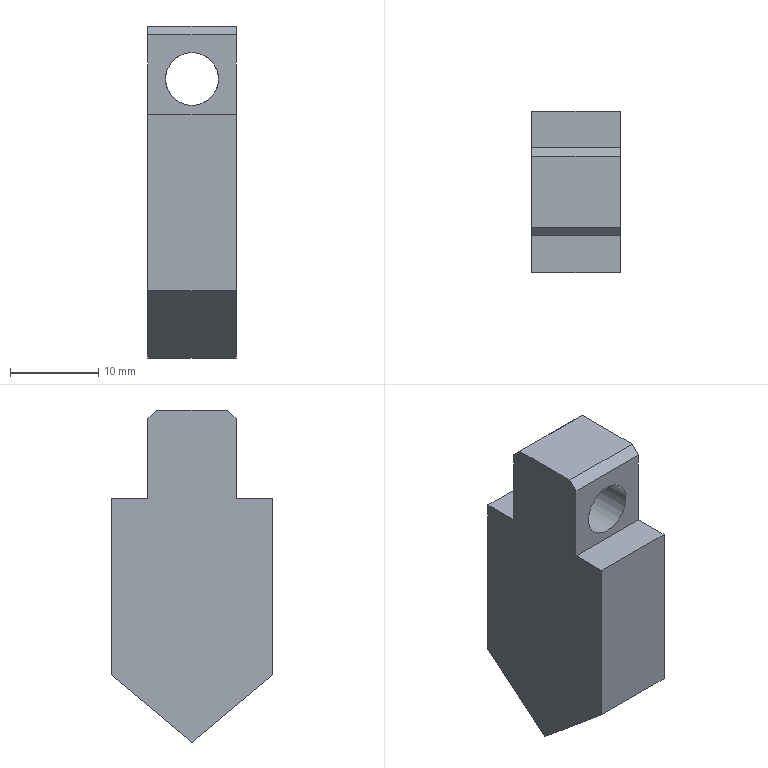Part | NX | features DATUM_CSYS 3, CHAMFER 2, EXTRUDE 2, SKETCH 2 | 1 solid | 14 faces | box 10 x 18.2 x 37.6 mm | volume 5039 mm3 | plane 13 | cylinder 1 | commonest cylinder face diameters 6 x1
STEP:
#1=CARTESIAN_POINT('',(0.,-9.1,27.6));
#2=VERTEX_POINT('',#1);
#3=CARTESIAN_POINT('',(0.,-9.1,7.6));
#4=VERTEX_POINT('',#3);
#5=CARTESIAN_POINT('',(0.,-9.1,27.6));
#6=DIRECTION('',(0.,0.,-1.));
#7=VECTOR('',#6,1000.);
#8=LINE('',#5,#7);
#9=EDGE_CURVE('',#2,#4,#8,.T.);
#10=ORIENTED_EDGE('',*,*,#9,.T.);
#11=CARTESIAN_POINT('',(10.,-9.1,7.6));
#12=VERTEX_POINT('',#11);
#13=CARTESIAN_POINT('',(10.,-9.1,7.6));
#14=DIRECTION('',(-1.,0.,0.));
#15=VECTOR('',#14,1000.);
#16=LINE('',#13,#15);
#17=EDGE_CURVE('',#12,#4,#16,.T.);
#18=ORIENTED_EDGE('',*,*,#17,.F.);
#19=CARTESIAN_POINT('',(10.,-9.1,27.6));
#20=VERTEX_POINT('',#19);
#21=CARTESIAN_POINT('',(10.,-9.1,27.6));
#22=DIRECTION('',(0.,0.,-1.));
#23=VECTOR('',#22,1000.);
#24=LINE('',#21,#23);
#25=EDGE_CURVE('',#20,#12,#24,.T.);
#26=ORIENTED_EDGE('',*,*,#25,.F.);
#27=CARTESIAN_POINT('',(10.,-9.1,27.6));
#28=DIRECTION('',(-1.,0.,0.));
#29=VECTOR('',#28,1000.);
#30=LINE('',#27,#29);
#31=EDGE_CURVE('',#20,#2,#30,.T.);
#32=ORIENTED_EDGE('',*,*,#31,.T.);
#33=EDGE_LOOP('',(#10,#18,#26,#32));
#34=FACE_BOUND('',#33,.T.);
#35=CARTESIAN_POINT('',(10.,-9.1,27.6));
#36=DIRECTION('',(0.,1.,0.));
#37=DIRECTION('',(0.,0.,1.));
#38=AXIS2_PLACEMENT_3D('',#35,#36,#37);
#39=PLANE('',#38);
#40=ADVANCED_FACE('',(#34),#39,.F.);
#41=CARTESIAN_POINT('',(0.,0.,0.));
#42=VERTEX_POINT('',#41);
#43=CARTESIAN_POINT('',(0.,-9.1,7.6));
#44=DIRECTION('',(0.,0.7675,-0.641));
#45=VECTOR('',#44,1000.);
#46=LINE('',#43,#45);
#47=EDGE_CURVE('',#4,#42,#46,.T.);
#48=ORIENTED_EDGE('',*,*,#47,.T.);
#49=CARTESIAN_POINT('',(10.,0.,0.));
#50=VERTEX_POINT('',#49);
#51=CARTESIAN_POINT('',(10.,0.,0.));
#52=DIRECTION('',(-1.,0.,0.));
#53=VECTOR('',#52,1000.);
#54=LINE('',#51,#53);
#55=EDGE_CURVE('',#50,#42,#54,.T.);
#56=ORIENTED_EDGE('',*,*,#55,.F.);
#57=CARTESIAN_POINT('',(10.,-9.1,7.6));
#58=DIRECTION('',(0.,0.7675,-0.641));
#59=VECTOR('',#58,1000.);
#60=LINE('',#57,#59);
#61=EDGE_CURVE('',#12,#50,#60,.T.);
#62=ORIENTED_EDGE('',*,*,#61,.F.);
#63=ORIENTED_EDGE('',*,*,#17,.T.);
#64=EDGE_LOOP('',(#48,#56,#62,#63));
#65=FACE_BOUND('',#64,.T.);
#66=CARTESIAN_POINT('',(10.,-9.1,7.6));
#67=DIRECTION('',(0.,0.641,0.7675));
#68=DIRECTION('',(0.,-0.7675,0.641));
#69=AXIS2_PLACEMENT_3D('',#66,#67,#68);
#70=PLANE('',#69);
#71=ADVANCED_FACE('',(#65),#70,.F.);
#72=CARTESIAN_POINT('',(0.,9.1,7.6));
#73=VERTEX_POINT('',#72);
#74=CARTESIAN_POINT('',(0.,0.,0.));
#75=DIRECTION('',(0.,0.7675,0.641));
#76=VECTOR('',#75,1000.);
#77=LINE('',#74,#76);
#78=EDGE_CURVE('',#42,#73,#77,.T.);
#79=ORIENTED_EDGE('',*,*,#78,.T.);
#80=CARTESIAN_POINT('',(10.,9.1,7.6));
#81=VERTEX_POINT('',#80);
#82=CARTESIAN_POINT('',(10.,9.1,7.6));
#83=DIRECTION('',(-1.,0.,0.));
#84=VECTOR('',#83,1000.);
#85=LINE('',#82,#84);
#86=EDGE_CURVE('',#81,#73,#85,.T.);
#87=ORIENTED_EDGE('',*,*,#86,.F.);
#88=CARTESIAN_POINT('',(10.,0.,0.));
#89=DIRECTION('',(0.,0.7675,0.641));
#90=VECTOR('',#89,1000.);
#91=LINE('',#88,#90);
#92=EDGE_CURVE('',#50,#81,#91,.T.);
#93=ORIENTED_EDGE('',*,*,#92,.F.);
#94=ORIENTED_EDGE('',*,*,#55,.T.);
#95=EDGE_LOOP('',(#79,#87,#93,#94));
#96=FACE_BOUND('',#95,.T.);
#97=CARTESIAN_POINT('',(10.,0.,0.));
#98=DIRECTION('',(0.,-0.641,0.7675));
#99=DIRECTION('',(0.,-0.7675,-0.641));
#100=AXIS2_PLACEMENT_3D('',#97,#98,#99);
#101=PLANE('',#100);
#102=ADVANCED_FACE('',(#96),#101,.F.);
#103=CARTESIAN_POINT('',(0.,9.1,27.6));
#104=VERTEX_POINT('',#103);
#105=CARTESIAN_POINT('',(0.,9.1,7.6));
#106=DIRECTION('',(0.,0.,1.));
#107=VECTOR('',#106,1000.);
#108=LINE('',#105,#107);
#109=EDGE_CURVE('',#73,#104,#108,.T.);
#110=ORIENTED_EDGE('',*,*,#109,.T.);
#111=CARTESIAN_POINT('',(10.,9.1,27.6));
#112=VERTEX_POINT('',#111);
#113=CARTESIAN_POINT('',(10.,9.1,27.6));
#114=DIRECTION('',(-1.,0.,0.));
#115=VECTOR('',#114,1000.);
#116=LINE('',#113,#115);
#117=EDGE_CURVE('',#112,#104,#116,.T.);
#118=ORIENTED_EDGE('',*,*,#117,.F.);
#119=CARTESIAN_POINT('',(10.,9.1,7.6));
#120=DIRECTION('',(0.,0.,1.));
#121=VECTOR('',#120,1000.);
#122=LINE('',#119,#121);
#123=EDGE_CURVE('',#81,#112,#122,.T.);
#124=ORIENTED_EDGE('',*,*,#123,.F.);
#125=ORIENTED_EDGE('',*,*,#86,.T.);
#126=EDGE_LOOP('',(#110,#118,#124,#125));
#127=FACE_BOUND('',#126,.T.);
#128=CARTESIAN_POINT('',(10.,9.1,7.6));
#129=DIRECTION('',(0.,-1.,0.));
#130=DIRECTION('',(0.,0.,-1.));
#131=AXIS2_PLACEMENT_3D('',#128,#129,#130);
#132=PLANE('',#131);
#133=ADVANCED_FACE('',(#127),#132,.F.);
#134=CARTESIAN_POINT('',(0.,5.,27.6));
#135=VERTEX_POINT('',#134);
#136=CARTESIAN_POINT('',(0.,9.1,27.6));
#137=DIRECTION('',(0.,-1.,0.));
#138=VECTOR('',#137,1000.);
#139=LINE('',#136,#138);
#140=EDGE_CURVE('',#104,#135,#139,.T.);
#141=ORIENTED_EDGE('',*,*,#140,.T.);
#142=CARTESIAN_POINT('',(10.,5.,27.6));
#143=VERTEX_POINT('',#142);
#144=CARTESIAN_POINT('',(10.,5.,27.6));
#145=DIRECTION('',(-1.,0.,0.));
#146=VECTOR('',#145,1000.);
#147=LINE('',#144,#146);
#148=EDGE_CURVE('',#143,#135,#147,.T.);
#149=ORIENTED_EDGE('',*,*,#148,.F.);
#150=CARTESIAN_POINT('',(10.,9.1,27.6));
#151=DIRECTION('',(0.,-1.,0.));
#152=VECTOR('',#151,1000.);
#153=LINE('',#150,#152);
#154=EDGE_CURVE('',#112,#143,#153,.T.);
#155=ORIENTED_EDGE('',*,*,#154,.F.);
#156=ORIENTED_EDGE('',*,*,#117,.T.);
#157=EDGE_LOOP('',(#141,#149,#155,#156));
#158=FACE_BOUND('',#157,.T.);
#159=CARTESIAN_POINT('',(10.,9.1,27.6));
#160=DIRECTION('',(0.,0.,-1.));
#161=DIRECTION('',(-1.,0.,0.));
#162=AXIS2_PLACEMENT_3D('',#159,#160,#161);
#163=PLANE('',#162);
#164=ADVANCED_FACE('',(#158),#163,.F.);
#165=CARTESIAN_POINT('',(2.,5.,31.6));
#166=VERTEX_POINT('',#165);
#167=CARTESIAN_POINT('',(5.,5.,31.6));
#168=DIRECTION('',(0.,1.,0.));
#169=DIRECTION('',(-1.,0.,0.));
#170=AXIS2_PLACEMENT_3D('',#167,#168,#169);
#171=CIRCLE('',#170,3.);
#172=EDGE_CURVE('',#166,#166,#171,.T.);
#173=ORIENTED_EDGE('',*,*,#172,.F.);
#174=EDGE_LOOP('',(#173));
#175=FACE_BOUND('',#174,.T.);
#176=CARTESIAN_POINT('',(0.,5.,36.6));
#177=VERTEX_POINT('',#176);
#178=CARTESIAN_POINT('',(0.,5.,27.6));
#179=DIRECTION('',(0.,0.,1.));
#180=VECTOR('',#179,1000.);
#181=LINE('',#178,#180);
#182=EDGE_CURVE('',#135,#177,#181,.T.);
#183=ORIENTED_EDGE('',*,*,#182,.T.);
#184=CARTESIAN_POINT('',(10.,5.,36.6));
#185=VERTEX_POINT('',#184);
#186=CARTESIAN_POINT('',(10.,5.,36.6));
#187=DIRECTION('',(1.,0.,0.));
#188=VECTOR('',#187,1000.);
#189=LINE('',#186,#188);
#190=EDGE_CURVE('',#177,#185,#189,.T.);
#191=ORIENTED_EDGE('',*,*,#190,.T.);
#192=CARTESIAN_POINT('',(10.,5.,27.6));
#193=DIRECTION('',(0.,0.,1.));
#194=VECTOR('',#193,1000.);
#195=LINE('',#192,#194);
#196=EDGE_CURVE('',#143,#185,#195,.T.);
#197=ORIENTED_EDGE('',*,*,#196,.F.);
#198=ORIENTED_EDGE('',*,*,#148,.T.);
#199=EDGE_LOOP('',(#183,#191,#197,#198));
#200=FACE_BOUND('',#199,.T.);
#201=CARTESIAN_POINT('',(10.,5.,27.6));
#202=DIRECTION('',(0.,-1.,0.));
#203=DIRECTION('',(0.,0.,-1.));
#204=AXIS2_PLACEMENT_3D('',#201,#202,#203);
#205=PLANE('',#204);
#206=ADVANCED_FACE('',(#175,#200),#205,.F.);
#207=CARTESIAN_POINT('',(0.,4.,37.6));
#208=VERTEX_POINT('',#207);
#209=CARTESIAN_POINT('',(0.,-4.,37.6));
#210=VERTEX_POINT('',#209);
#211=CARTESIAN_POINT('',(0.,0.,37.6));
#212=DIRECTION('',(0.,-1.,0.));
#213=VECTOR('',#212,1000.);
#214=LINE('',#211,#213);
#215=EDGE_CURVE('',#208,#210,#214,.T.);
#216=ORIENTED_EDGE('',*,*,#215,.T.);
#217=CARTESIAN_POINT('',(10.,-4.,37.6));
#218=VERTEX_POINT('',#217);
#219=CARTESIAN_POINT('',(10.,-4.,37.6));
#220=DIRECTION('',(1.,0.,0.));
#221=VECTOR('',#220,1000.);
#222=LINE('',#219,#221);
#223=EDGE_CURVE('',#210,#218,#222,.T.);
#224=ORIENTED_EDGE('',*,*,#223,.T.);
#225=CARTESIAN_POINT('',(10.,4.,37.6));
#226=VERTEX_POINT('',#225);
#227=CARTESIAN_POINT('',(10.,5.,37.6));
#228=DIRECTION('',(0.,-1.,0.));
#229=VECTOR('',#228,1000.);
#230=LINE('',#227,#229);
#231=EDGE_CURVE('',#226,#218,#230,.T.);
#232=ORIENTED_EDGE('',*,*,#231,.F.);
#233=CARTESIAN_POINT('',(10.,4.,37.6));
#234=DIRECTION('',(-1.,0.,0.));
#235=VECTOR('',#234,1000.);
#236=LINE('',#233,#235);
#237=EDGE_CURVE('',#226,#208,#236,.T.);
#238=ORIENTED_EDGE('',*,*,#237,.T.);
#239=EDGE_LOOP('',(#216,#224,#232,#238));
#240=FACE_BOUND('',#239,.T.);
#241=CARTESIAN_POINT('',(10.,0.,37.6));
#242=DIRECTION('',(0.,0.,-1.));
#243=DIRECTION('',(-1.,0.,0.));
#244=AXIS2_PLACEMENT_3D('',#241,#242,#243);
#245=PLANE('',#244);
#246=ADVANCED_FACE('',(#240),#245,.F.);
#247=CARTESIAN_POINT('',(5.,-5.,34.6));
#248=VERTEX_POINT('',#247);
#249=CARTESIAN_POINT('',(5.,-5.,31.6));
#250=DIRECTION('',(0.,1.,0.));
#251=DIRECTION('',(0.,0.,1.));
#252=AXIS2_PLACEMENT_3D('',#249,#250,#251);
#253=CIRCLE('',#252,3.);
#254=EDGE_CURVE('',#248,#248,#253,.T.);
#255=ORIENTED_EDGE('',*,*,#254,.T.);
#256=EDGE_LOOP('',(#255));
#257=FACE_BOUND('',#256,.T.);
#258=CARTESIAN_POINT('',(10.,-5.,36.6));
#259=VERTEX_POINT('',#258);
#260=CARTESIAN_POINT('',(10.,-5.,27.6));
#261=VERTEX_POINT('',#260);
#262=CARTESIAN_POINT('',(10.,-5.,37.6));
#263=DIRECTION('',(0.,0.,-1.));
#264=VECTOR('',#263,1000.);
#265=LINE('',#262,#264);
#266=EDGE_CURVE('',#259,#261,#265,.T.);
#267=ORIENTED_EDGE('',*,*,#266,.F.);
#268=CARTESIAN_POINT('',(0.,-5.,36.6));
#269=VERTEX_POINT('',#268);
#270=CARTESIAN_POINT('',(10.,-5.,36.6));
#271=DIRECTION('',(-1.,0.,0.));
#272=VECTOR('',#271,1000.);
#273=LINE('',#270,#272);
#274=EDGE_CURVE('',#259,#269,#273,.T.);
#275=ORIENTED_EDGE('',*,*,#274,.T.);
#276=CARTESIAN_POINT('',(0.,-5.,27.6));
#277=VERTEX_POINT('',#276);
#278=CARTESIAN_POINT('',(0.,-5.,37.6));
#279=DIRECTION('',(0.,0.,-1.));
#280=VECTOR('',#279,1000.);
#281=LINE('',#278,#280);
#282=EDGE_CURVE('',#269,#277,#281,.T.);
#283=ORIENTED_EDGE('',*,*,#282,.T.);
#284=CARTESIAN_POINT('',(10.,-5.,27.6));
#285=DIRECTION('',(-1.,0.,0.));
#286=VECTOR('',#285,1000.);
#287=LINE('',#284,#286);
#288=EDGE_CURVE('',#261,#277,#287,.T.);
#289=ORIENTED_EDGE('',*,*,#288,.F.);
#290=EDGE_LOOP('',(#267,#275,#283,#289));
#291=FACE_BOUND('',#290,.T.);
#292=CARTESIAN_POINT('',(10.,-5.,37.6));
#293=DIRECTION('',(0.,1.,0.));
#294=DIRECTION('',(0.,0.,1.));
#295=AXIS2_PLACEMENT_3D('',#292,#293,#294);
#296=PLANE('',#295);
#297=ADVANCED_FACE('',(#257,#291),#296,.F.);
#298=CARTESIAN_POINT('',(0.,-5.,27.6));
#299=DIRECTION('',(0.,-1.,0.));
#300=VECTOR('',#299,1000.);
#301=LINE('',#298,#300);
#302=EDGE_CURVE('',#277,#2,#301,.T.);
#303=ORIENTED_EDGE('',*,*,#302,.T.);
#304=ORIENTED_EDGE('',*,*,#31,.F.);
#305=CARTESIAN_POINT('',(10.,-5.,27.6));
#306=DIRECTION('',(0.,-1.,0.));
#307=VECTOR('',#306,1000.);
#308=LINE('',#305,#307);
#309=EDGE_CURVE('',#261,#20,#308,.T.);
#310=ORIENTED_EDGE('',*,*,#309,.F.);
#311=ORIENTED_EDGE('',*,*,#288,.T.);
#312=EDGE_LOOP('',(#303,#304,#310,#311));
#313=FACE_BOUND('',#312,.T.);
#314=CARTESIAN_POINT('',(10.,-5.,27.6));
#315=DIRECTION('',(0.,0.,-1.));
#316=DIRECTION('',(-1.,0.,0.));
#317=AXIS2_PLACEMENT_3D('',#314,#315,#316);
#318=PLANE('',#317);
#319=ADVANCED_FACE('',(#313),#318,.F.);
#320=ORIENTED_EDGE('',*,*,#231,.T.);
#321=CARTESIAN_POINT('',(10.,-5.,36.6));
#322=DIRECTION('',(0.,0.7071,0.7071));
#323=VECTOR('',#322,1000.);
#324=LINE('',#321,#323);
#325=EDGE_CURVE('',#218,#259,#324,.F.);
#326=ORIENTED_EDGE('',*,*,#325,.T.);
#327=ORIENTED_EDGE('',*,*,#266,.T.);
#328=ORIENTED_EDGE('',*,*,#309,.T.);
#329=ORIENTED_EDGE('',*,*,#25,.T.);
#330=ORIENTED_EDGE('',*,*,#61,.T.);
#331=ORIENTED_EDGE('',*,*,#92,.T.);
#332=ORIENTED_EDGE('',*,*,#123,.T.);
#333=ORIENTED_EDGE('',*,*,#154,.T.);
#334=ORIENTED_EDGE('',*,*,#196,.T.);
#335=CARTESIAN_POINT('',(10.,4.,37.6));
#336=DIRECTION('',(0.,0.7071,-0.7071));
#337=VECTOR('',#336,1000.);
#338=LINE('',#335,#337);
#339=EDGE_CURVE('',#185,#226,#338,.F.);
#340=ORIENTED_EDGE('',*,*,#339,.T.);
#341=EDGE_LOOP('',(#320,#326,#327,#328,#329,#330,#331,#332,#333,#334,#340));
#342=FACE_BOUND('',#341,.T.);
#343=CARTESIAN_POINT('',(10.,0.,0.));
#344=DIRECTION('',(-1.,0.,0.));
#345=DIRECTION('',(0.,0.,1.));
#346=AXIS2_PLACEMENT_3D('',#343,#344,#345);
#347=PLANE('',#346);
#348=ADVANCED_FACE('',(#342),#347,.F.);
#349=ORIENTED_EDGE('',*,*,#282,.F.);
#350=CARTESIAN_POINT('',(0.,-20.8,20.8));
#351=DIRECTION('',(0.,-0.7071,-0.7071));
#352=VECTOR('',#351,1000.);
#353=LINE('',#350,#352);
#354=EDGE_CURVE('',#269,#210,#353,.F.);
#355=ORIENTED_EDGE('',*,*,#354,.T.);
#356=ORIENTED_EDGE('',*,*,#215,.F.);
#357=CARTESIAN_POINT('',(0.,20.8,20.8));
#358=DIRECTION('',(0.,-0.7071,0.7071));
#359=VECTOR('',#358,1000.);
#360=LINE('',#357,#359);
#361=EDGE_CURVE('',#208,#177,#360,.F.);
#362=ORIENTED_EDGE('',*,*,#361,.T.);
#363=ORIENTED_EDGE('',*,*,#182,.F.);
#364=ORIENTED_EDGE('',*,*,#140,.F.);
#365=ORIENTED_EDGE('',*,*,#109,.F.);
#366=ORIENTED_EDGE('',*,*,#78,.F.);
#367=ORIENTED_EDGE('',*,*,#47,.F.);
#368=ORIENTED_EDGE('',*,*,#9,.F.);
#369=ORIENTED_EDGE('',*,*,#302,.F.);
#370=EDGE_LOOP('',(#349,#355,#356,#362,#363,#364,#365,#366,#367,#368,#369));
#371=FACE_BOUND('',#370,.T.);
#372=CARTESIAN_POINT('',(0.,0.,0.));
#373=DIRECTION('',(-1.,0.,0.));
#374=DIRECTION('',(0.,0.,1.));
#375=AXIS2_PLACEMENT_3D('',#372,#373,#374);
#376=PLANE('',#375);
#377=ADVANCED_FACE('',(#371),#376,.T.);
#378=ORIENTED_EDGE('',*,*,#339,.F.);
#379=ORIENTED_EDGE('',*,*,#190,.F.);
#380=ORIENTED_EDGE('',*,*,#361,.F.);
#381=ORIENTED_EDGE('',*,*,#237,.F.);
#382=EDGE_LOOP('',(#378,#379,#380,#381));
#383=FACE_BOUND('',#382,.T.);
#384=CARTESIAN_POINT('',(10.,4.,37.6));
#385=DIRECTION('',(0.,-0.7071,-0.7071));
#386=DIRECTION('',(-1.,0.,0.));
#387=AXIS2_PLACEMENT_3D('',#384,#385,#386);
#388=PLANE('',#387);
#389=ADVANCED_FACE('',(#383),#388,.F.);
#390=ORIENTED_EDGE('',*,*,#325,.F.);
#391=ORIENTED_EDGE('',*,*,#223,.F.);
#392=ORIENTED_EDGE('',*,*,#354,.F.);
#393=ORIENTED_EDGE('',*,*,#274,.F.);
#394=EDGE_LOOP('',(#390,#391,#392,#393));
#395=FACE_BOUND('',#394,.T.);
#396=CARTESIAN_POINT('',(10.,-5.,36.6));
#397=DIRECTION('',(0.,0.7071,-0.7071));
#398=DIRECTION('',(-1.,0.,0.));
#399=AXIS2_PLACEMENT_3D('',#396,#397,#398);
#400=PLANE('',#399);
#401=ADVANCED_FACE('',(#395),#400,.F.);
#402=ORIENTED_EDGE('',*,*,#172,.T.);
#403=EDGE_LOOP('',(#402));
#404=FACE_BOUND('',#403,.T.);
#405=ORIENTED_EDGE('',*,*,#254,.F.);
#406=EDGE_LOOP('',(#405));
#407=FACE_BOUND('',#406,.T.);
#408=CARTESIAN_POINT('',(5.,-13.,31.6));
#409=DIRECTION('',(0.,1.,0.));
#410=DIRECTION('',(0.,0.,1.));
#411=AXIS2_PLACEMENT_3D('',#408,#409,#410);
#412=CYLINDRICAL_SURFACE('',#411,3.);
#413=ADVANCED_FACE('',(#404,#407),#412,.F.);
#414=CLOSED_SHELL('',(#40,#71,#102,#133,#164,#206,#246,#297,#319,#348,#377,#389,#401,#413));
#415=MANIFOLD_SOLID_BREP('',#414);
#416=(LENGTH_UNIT()NAMED_UNIT(*)SI_UNIT(.MILLI.,.METRE.));
#417=UNCERTAINTY_MEASURE_WITH_UNIT(LENGTH_MEASURE(0.00001),#416,'','');
#418=(NAMED_UNIT(*)PLANE_ANGLE_UNIT()SI_UNIT($,.RADIAN.));
#419=(NAMED_UNIT(*)SI_UNIT($,.STERADIAN.)SOLID_ANGLE_UNIT());
#420=(GEOMETRIC_REPRESENTATION_CONTEXT(3)GLOBAL_UNCERTAINTY_ASSIGNED_CONTEXT((#417))GLOBAL_UNIT_ASSIGNED_CONTEXT((#416,#418,#419))REPRESENTATION_CONTEXT('',''));
#421=ADVANCED_BREP_SHAPE_REPRESENTATION('',(#415),#420);